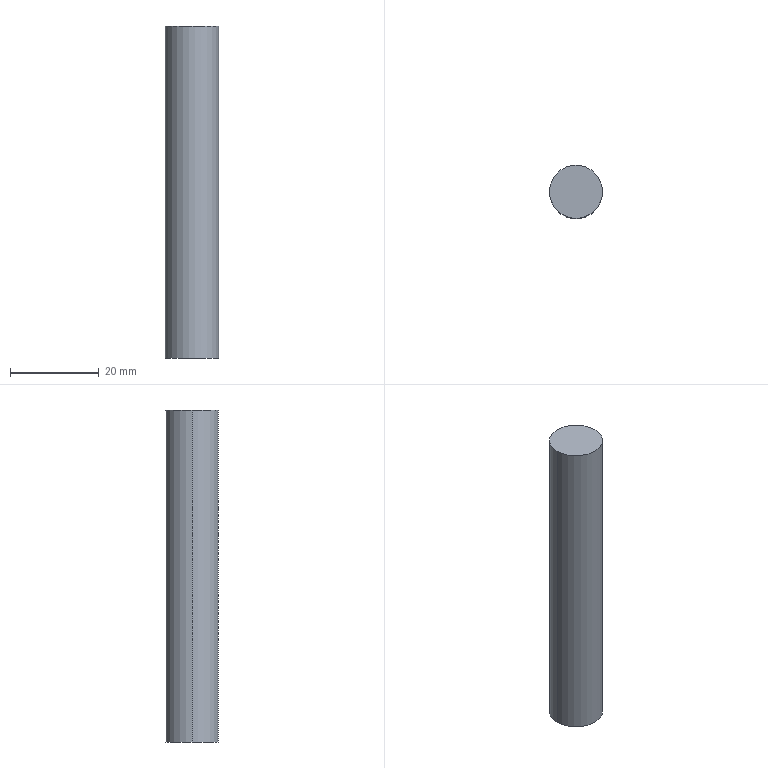Part | SolidWorks | features Extrusion 1 | 1 solid | 4 faces | box 12 x 12 x 75 mm | volume 8482 mm3 | cylinder 2 | plane 2 | commonest cylinder face diameters 12 x2
STEP:
#1=CARTESIAN_POINT('',(6.,0.,37.5));
#2=VERTEX_POINT('',#1);
#3=CARTESIAN_POINT('',(-6.,0.,37.5));
#4=VERTEX_POINT('',#3);
#5=CARTESIAN_POINT('',(0.,0.,37.5));
#6=DIRECTION('',(0.,0.,1.));
#7=DIRECTION('',(1.,0.,0.));
#8=AXIS2_PLACEMENT_3D('',#5,#6,#7);
#9=CIRCLE('',#8,6.);
#10=EDGE_CURVE('',#2,#4,#9,.T.);
#11=ORIENTED_EDGE('',*,*,#10,.F.);
#12=CARTESIAN_POINT('',(6.,0.,-37.5));
#13=VERTEX_POINT('',#12);
#14=CARTESIAN_POINT('',(6.,0.,37.5));
#15=DIRECTION('',(0.,0.,-1.));
#16=VECTOR('',#15,1000.);
#17=LINE('',#14,#16);
#18=EDGE_CURVE('',#2,#13,#17,.T.);
#19=ORIENTED_EDGE('',*,*,#18,.T.);
#20=CARTESIAN_POINT('',(-6.,0.,-37.5));
#21=VERTEX_POINT('',#20);
#22=CARTESIAN_POINT('',(0.,0.,-37.5));
#23=DIRECTION('',(0.,0.,1.));
#24=DIRECTION('',(1.,0.,0.));
#25=AXIS2_PLACEMENT_3D('',#22,#23,#24);
#26=CIRCLE('',#25,6.);
#27=EDGE_CURVE('',#13,#21,#26,.T.);
#28=ORIENTED_EDGE('',*,*,#27,.T.);
#29=CARTESIAN_POINT('',(-6.,0.,37.5));
#30=DIRECTION('',(0.,0.,-1.));
#31=VECTOR('',#30,1000.);
#32=LINE('',#29,#31);
#33=EDGE_CURVE('',#4,#21,#32,.T.);
#34=ORIENTED_EDGE('',*,*,#33,.F.);
#35=EDGE_LOOP('',(#11,#19,#28,#34));
#36=FACE_OUTER_BOUND('',#35,.T.);
#37=CARTESIAN_POINT('',(0.,0.,37.5));
#38=DIRECTION('',(0.,0.,-1.));
#39=DIRECTION('',(-1.,0.,0.));
#40=AXIS2_PLACEMENT_3D('',#37,#38,#39);
#41=CYLINDRICAL_SURFACE('',#40,6.);
#42=ADVANCED_FACE('',(#36),#41,.T.);
#43=ORIENTED_EDGE('',*,*,#18,.F.);
#44=CARTESIAN_POINT('',(0.,0.,37.5));
#45=DIRECTION('',(0.,0.,1.));
#46=DIRECTION('',(1.,0.,0.));
#47=AXIS2_PLACEMENT_3D('',#44,#45,#46);
#48=CIRCLE('',#47,6.);
#49=EDGE_CURVE('',#4,#2,#48,.T.);
#50=ORIENTED_EDGE('',*,*,#49,.F.);
#51=ORIENTED_EDGE('',*,*,#33,.T.);
#52=CARTESIAN_POINT('',(0.,0.,-37.5));
#53=DIRECTION('',(0.,0.,1.));
#54=DIRECTION('',(1.,0.,0.));
#55=AXIS2_PLACEMENT_3D('',#52,#53,#54);
#56=CIRCLE('',#55,6.);
#57=EDGE_CURVE('',#21,#13,#56,.T.);
#58=ORIENTED_EDGE('',*,*,#57,.T.);
#59=EDGE_LOOP('',(#43,#50,#51,#58));
#60=FACE_OUTER_BOUND('',#59,.T.);
#61=CARTESIAN_POINT('',(0.,0.,37.5));
#62=DIRECTION('',(0.,0.,-1.));
#63=DIRECTION('',(-1.,0.,0.));
#64=AXIS2_PLACEMENT_3D('',#61,#62,#63);
#65=CYLINDRICAL_SURFACE('',#64,6.);
#66=ADVANCED_FACE('',(#60),#65,.T.);
#67=ORIENTED_EDGE('',*,*,#49,.T.);
#68=ORIENTED_EDGE('',*,*,#10,.T.);
#69=EDGE_LOOP('',(#67,#68));
#70=FACE_OUTER_BOUND('',#69,.T.);
#71=CARTESIAN_POINT('',(0.,0.,37.5));
#72=DIRECTION('',(0.,0.,1.));
#73=DIRECTION('',(1.,0.,0.));
#74=AXIS2_PLACEMENT_3D('',#71,#72,#73);
#75=PLANE('',#74);
#76=ADVANCED_FACE('',(#70),#75,.T.);
#77=ORIENTED_EDGE('',*,*,#57,.F.);
#78=ORIENTED_EDGE('',*,*,#27,.F.);
#79=EDGE_LOOP('',(#77,#78));
#80=FACE_OUTER_BOUND('',#79,.T.);
#81=CARTESIAN_POINT('',(0.,0.,-37.5));
#82=DIRECTION('',(0.,0.,1.));
#83=DIRECTION('',(1.,0.,0.));
#84=AXIS2_PLACEMENT_3D('',#81,#82,#83);
#85=PLANE('',#84);
#86=ADVANCED_FACE('',(#80),#85,.F.);
#87=CLOSED_SHELL('',(#42,#66,#76,#86));
#88=MANIFOLD_SOLID_BREP('',#87);
#89=CARTESIAN_POINT('',(0.,0.,0.));
#90=DIRECTION('',(0.,0.,1.));
#91=DIRECTION('',(1.,0.,0.));
#92=AXIS2_PLACEMENT_3D('',#89,#90,#91);
#93=(LENGTH_UNIT()NAMED_UNIT(*)SI_UNIT(.MILLI.,.METRE.));
#94=UNCERTAINTY_MEASURE_WITH_UNIT(LENGTH_MEASURE(0.00001),#93,'','');
#95=(NAMED_UNIT(*)PLANE_ANGLE_UNIT()SI_UNIT($,.RADIAN.));
#96=(NAMED_UNIT(*)SI_UNIT($,.STERADIAN.)SOLID_ANGLE_UNIT());
#97=(GEOMETRIC_REPRESENTATION_CONTEXT(3)GLOBAL_UNCERTAINTY_ASSIGNED_CONTEXT((#94))GLOBAL_UNIT_ASSIGNED_CONTEXT((#93,#95,#96))REPRESENTATION_CONTEXT('',''));
#98=ADVANCED_BREP_SHAPE_REPRESENTATION('',(#88,#92),#97);